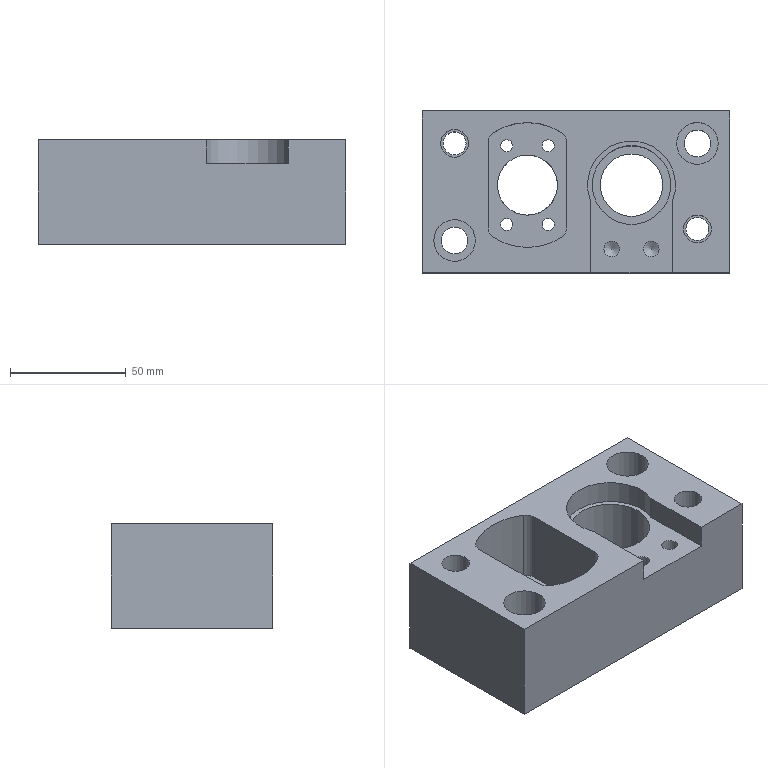Part | NX | features 26 2 | 1 solid | 43 faces | box 133 x 70 x 45 mm | volume 282044 mm3 | cylinder 24 | plane 17 | cone 2 | commonest cylinder face diameters 5.2 x4 10 x4 6.8 x2 10.001 x2 11.5 x2 12 x2
STEP:
#1=CARTESIAN_POINT('',(2251.6,-38.,-78.));
#2=VERTEX_POINT('',#1);
#3=CARTESIAN_POINT('',(2251.6,-7.158,-78.));
#4=VERTEX_POINT('',#3);
#5=CARTESIAN_POINT('',(2251.6,-13.,-78.));
#6=DIRECTION('',(0.,1.,0.));
#7=VECTOR('',#6,1000.);
#8=LINE('',#5,#7);
#9=EDGE_CURVE('',#2,#4,#8,.T.);
#10=ORIENTED_EDGE('',*,*,#9,.T.);
#11=CARTESIAN_POINT('',(2216.4,-7.158,-78.));
#12=VERTEX_POINT('',#11);
#13=CARTESIAN_POINT('',(2234.,0.,-78.));
#14=DIRECTION('',(0.,0.,1.));
#15=DIRECTION('',(-1.,0.,0.));
#16=AXIS2_PLACEMENT_3D('',#13,#14,#15);
#17=CIRCLE('',#16,19.);
#18=EDGE_CURVE('',#4,#12,#17,.T.);
#19=ORIENTED_EDGE('',*,*,#18,.T.);
#20=CARTESIAN_POINT('',(2216.4,-38.,-78.));
#21=VERTEX_POINT('',#20);
#22=CARTESIAN_POINT('',(2216.4,-13.,-78.));
#23=DIRECTION('',(0.,-1.,0.));
#24=VECTOR('',#23,1000.);
#25=LINE('',#22,#24);
#26=EDGE_CURVE('',#12,#21,#25,.T.);
#27=ORIENTED_EDGE('',*,*,#26,.T.);
#28=CARTESIAN_POINT('',(2234.,-38.,-78.));
#29=DIRECTION('',(1.,0.,0.));
#30=VECTOR('',#29,1000.);
#31=LINE('',#28,#30);
#32=EDGE_CURVE('',#21,#2,#31,.T.);
#33=ORIENTED_EDGE('',*,*,#32,.T.);
#34=EDGE_LOOP('',(#10,#19,#27,#33));
#35=FACE_BOUND('',#34,.T.);
#36=CARTESIAN_POINT('',(2239.1,-27.7,-78.));
#37=VERTEX_POINT('',#36);
#38=CARTESIAN_POINT('',(2242.5,-27.7,-78.));
#39=DIRECTION('',(0.,0.,-1.));
#40=DIRECTION('',(-1.,0.,0.));
#41=AXIS2_PLACEMENT_3D('',#38,#39,#40);
#42=CIRCLE('',#41,3.4);
#43=EDGE_CURVE('',#37,#37,#42,.T.);
#44=ORIENTED_EDGE('',*,*,#43,.T.);
#45=EDGE_LOOP('',(#44));
#46=FACE_BOUND('',#45,.T.);
#47=CARTESIAN_POINT('',(2222.1,-27.7,-78.));
#48=VERTEX_POINT('',#47);
#49=CARTESIAN_POINT('',(2225.5,-27.7,-78.));
#50=DIRECTION('',(0.,0.,1.));
#51=DIRECTION('',(-1.,0.,0.));
#52=AXIS2_PLACEMENT_3D('',#49,#50,#51);
#53=CIRCLE('',#52,3.4);
#54=EDGE_CURVE('',#48,#48,#53,.T.);
#55=ORIENTED_EDGE('',*,*,#54,.F.);
#56=EDGE_LOOP('',(#55));
#57=FACE_BOUND('',#56,.T.);
#58=CARTESIAN_POINT('',(2217.,0.,-78.));
#59=VERTEX_POINT('',#58);
#60=CARTESIAN_POINT('',(2234.,0.,-78.));
#61=DIRECTION('',(0.,0.,1.));
#62=DIRECTION('',(-1.,0.,0.));
#63=AXIS2_PLACEMENT_3D('',#60,#61,#62);
#64=CIRCLE('',#63,17.);
#65=EDGE_CURVE('',#59,#59,#64,.T.);
#66=ORIENTED_EDGE('',*,*,#65,.F.);
#67=EDGE_LOOP('',(#66));
#68=FACE_BOUND('',#67,.T.);
#69=CARTESIAN_POINT('',(2258.,-3.,-78.));
#70=DIRECTION('',(0.,0.,1.));
#71=DIRECTION('',(1.,0.,0.));
#72=AXIS2_PLACEMENT_3D('',#69,#70,#71);
#73=PLANE('',#72);
#74=ADVANCED_FACE('',(#35,#46,#57,#68),#73,.T.);
#75=CARTESIAN_POINT('',(2217.,0.,-108.));
#76=VERTEX_POINT('',#75);
#77=CARTESIAN_POINT('',(2234.,0.,-108.));
#78=DIRECTION('',(0.,0.,-1.));
#79=DIRECTION('',(-1.,0.,0.));
#80=AXIS2_PLACEMENT_3D('',#77,#78,#79);
#81=CIRCLE('',#80,17.);
#82=EDGE_CURVE('',#76,#76,#81,.T.);
#83=ORIENTED_EDGE('',*,*,#82,.T.);
#84=EDGE_LOOP('',(#83));
#85=FACE_BOUND('',#84,.T.);
#86=ORIENTED_EDGE('',*,*,#65,.T.);
#87=EDGE_LOOP('',(#86));
#88=FACE_BOUND('',#87,.T.);
#89=CARTESIAN_POINT('',(2234.,0.,512.));
#90=DIRECTION('',(0.,0.,-1.));
#91=DIRECTION('',(-1.,0.,0.));
#92=AXIS2_PLACEMENT_3D('',#89,#90,#91);
#93=CYLINDRICAL_SURFACE('',#92,17.);
#94=ADVANCED_FACE('',(#85,#88),#93,.F.);
#95=CARTESIAN_POINT('',(2151.5,18.,-68.));
#96=VERTEX_POINT('',#95);
#97=CARTESIAN_POINT('',(2157.5,18.,-68.));
#98=DIRECTION('',(0.,0.,1.));
#99=DIRECTION('',(-1.,0.,0.));
#100=AXIS2_PLACEMENT_3D('',#97,#98,#99);
#101=CIRCLE('',#100,6.);
#102=EDGE_CURVE('',#96,#96,#101,.T.);
#103=ORIENTED_EDGE('',*,*,#102,.F.);
#104=EDGE_LOOP('',(#103));
#105=FACE_BOUND('',#104,.T.);
#106=CARTESIAN_POINT('',(2256.5,-19.,-68.));
#107=VERTEX_POINT('',#106);
#108=CARTESIAN_POINT('',(2262.5,-19.,-68.));
#109=DIRECTION('',(0.,0.,1.));
#110=DIRECTION('',(-1.,0.,0.));
#111=AXIS2_PLACEMENT_3D('',#108,#109,#110);
#112=CIRCLE('',#111,6.);
#113=EDGE_CURVE('',#107,#107,#112,.T.);
#114=ORIENTED_EDGE('',*,*,#113,.F.);
#115=EDGE_LOOP('',(#114));
#116=FACE_BOUND('',#115,.T.);
#117=CARTESIAN_POINT('',(2253.5,18.,-68.));
#118=VERTEX_POINT('',#117);
#119=CARTESIAN_POINT('',(2262.5,18.,-68.));
#120=DIRECTION('',(0.,0.,-1.));
#121=DIRECTION('',(-1.,0.,0.));
#122=AXIS2_PLACEMENT_3D('',#119,#120,#121);
#123=CIRCLE('',#122,9.);
#124=EDGE_CURVE('',#118,#118,#123,.T.);
#125=ORIENTED_EDGE('',*,*,#124,.T.);
#126=EDGE_LOOP('',(#125));
#127=FACE_BOUND('',#126,.T.);
#128=CARTESIAN_POINT('',(2148.5,-24.,-68.));
#129=VERTEX_POINT('',#128);
#130=CARTESIAN_POINT('',(2157.5,-24.,-68.));
#131=DIRECTION('',(0.,0.,-1.));
#132=DIRECTION('',(-1.,0.,0.));
#133=AXIS2_PLACEMENT_3D('',#130,#131,#132);
#134=CIRCLE('',#133,9.);
#135=EDGE_CURVE('',#129,#129,#134,.T.);
#136=ORIENTED_EDGE('',*,*,#135,.T.);
#137=EDGE_LOOP('',(#136));
#138=FACE_BOUND('',#137,.T.);
#139=CARTESIAN_POINT('',(2206.,18.439,-68.));
#140=VERTEX_POINT('',#139);
#141=CARTESIAN_POINT('',(2206.,-18.439,-68.));
#142=VERTEX_POINT('',#141);
#143=CARTESIAN_POINT('',(2206.,211.,-68.));
#144=DIRECTION('',(0.,-1.,0.));
#145=VECTOR('',#144,1000.);
#146=LINE('',#143,#145);
#147=EDGE_CURVE('',#140,#142,#146,.T.);
#148=ORIENTED_EDGE('',*,*,#147,.T.);
#149=CARTESIAN_POINT('',(2203.727,-22.63,-68.));
#150=VERTEX_POINT('',#149);
#151=CARTESIAN_POINT('',(2201.,-18.439,-68.));
#152=DIRECTION('',(0.,0.,-1.));
#153=DIRECTION('',(-1.,0.,0.));
#154=AXIS2_PLACEMENT_3D('',#151,#152,#153);
#155=CIRCLE('',#154,5.);
#156=EDGE_CURVE('',#142,#150,#155,.T.);
#157=ORIENTED_EDGE('',*,*,#156,.T.);
#158=CARTESIAN_POINT('',(2174.273,-22.63,-68.));
#159=VERTEX_POINT('',#158);
#160=CARTESIAN_POINT('',(2189.,0.,-68.));
#161=DIRECTION('',(0.,0.,-1.));
#162=DIRECTION('',(-1.,0.,0.));
#163=AXIS2_PLACEMENT_3D('',#160,#161,#162);
#164=CIRCLE('',#163,27.);
#165=EDGE_CURVE('',#150,#159,#164,.T.);
#166=ORIENTED_EDGE('',*,*,#165,.T.);
#167=CARTESIAN_POINT('',(2172.,-18.439,-68.));
#168=VERTEX_POINT('',#167);
#169=CARTESIAN_POINT('',(2177.,-18.439,-68.));
#170=DIRECTION('',(0.,0.,-1.));
#171=DIRECTION('',(-1.,0.,0.));
#172=AXIS2_PLACEMENT_3D('',#169,#170,#171);
#173=CIRCLE('',#172,5.);
#174=EDGE_CURVE('',#159,#168,#173,.T.);
#175=ORIENTED_EDGE('',*,*,#174,.T.);
#176=CARTESIAN_POINT('',(2172.,18.439,-68.));
#177=VERTEX_POINT('',#176);
#178=CARTESIAN_POINT('',(2172.,211.,-68.));
#179=DIRECTION('',(0.,1.,0.));
#180=VECTOR('',#179,1000.);
#181=LINE('',#178,#180);
#182=EDGE_CURVE('',#168,#177,#181,.T.);
#183=ORIENTED_EDGE('',*,*,#182,.T.);
#184=CARTESIAN_POINT('',(2174.273,22.63,-68.));
#185=VERTEX_POINT('',#184);
#186=CARTESIAN_POINT('',(2177.,18.439,-68.));
#187=DIRECTION('',(0.,0.,-1.));
#188=DIRECTION('',(-1.,0.,0.));
#189=AXIS2_PLACEMENT_3D('',#186,#187,#188);
#190=CIRCLE('',#189,5.);
#191=EDGE_CURVE('',#177,#185,#190,.T.);
#192=ORIENTED_EDGE('',*,*,#191,.T.);
#193=CARTESIAN_POINT('',(2203.727,22.63,-68.));
#194=VERTEX_POINT('',#193);
#195=CARTESIAN_POINT('',(2189.,0.,-68.));
#196=DIRECTION('',(0.,0.,-1.));
#197=DIRECTION('',(-1.,0.,0.));
#198=AXIS2_PLACEMENT_3D('',#195,#196,#197);
#199=CIRCLE('',#198,27.);
#200=EDGE_CURVE('',#185,#194,#199,.T.);
#201=ORIENTED_EDGE('',*,*,#200,.T.);
#202=CARTESIAN_POINT('',(2201.,18.439,-68.));
#203=DIRECTION('',(0.,0.,-1.));
#204=DIRECTION('',(-1.,0.,0.));
#205=AXIS2_PLACEMENT_3D('',#202,#203,#204);
#206=CIRCLE('',#205,5.);
#207=EDGE_CURVE('',#194,#140,#206,.T.);
#208=ORIENTED_EDGE('',*,*,#207,.T.);
#209=EDGE_LOOP('',(#148,#157,#166,#175,#183,#192,#201,#208));
#210=FACE_BOUND('',#209,.T.);
#211=CARTESIAN_POINT('',(2216.4,-7.158,-68.));
#212=VERTEX_POINT('',#211);
#213=CARTESIAN_POINT('',(2251.6,-7.158,-68.));
#214=VERTEX_POINT('',#213);
#215=CARTESIAN_POINT('',(2234.,0.,-68.));
#216=DIRECTION('',(0.,0.,-1.));
#217=DIRECTION('',(1.,0.,0.));
#218=AXIS2_PLACEMENT_3D('',#215,#216,#217);
#219=CIRCLE('',#218,19.);
#220=EDGE_CURVE('',#212,#214,#219,.T.);
#221=ORIENTED_EDGE('',*,*,#220,.T.);
#222=CARTESIAN_POINT('',(2251.6,-38.,-68.));
#223=VERTEX_POINT('',#222);
#224=CARTESIAN_POINT('',(2251.6,206.,-68.));
#225=DIRECTION('',(0.,-1.,0.));
#226=VECTOR('',#225,1000.);
#227=LINE('',#224,#226);
#228=EDGE_CURVE('',#214,#223,#227,.T.);
#229=ORIENTED_EDGE('',*,*,#228,.T.);
#230=CARTESIAN_POINT('',(2276.5,-38.,-68.));
#231=VERTEX_POINT('',#230);
#232=CARTESIAN_POINT('',(2234.,-38.,-68.));
#233=DIRECTION('',(-1.,0.,0.));
#234=VECTOR('',#233,1000.);
#235=LINE('',#232,#234);
#236=EDGE_CURVE('',#231,#223,#235,.T.);
#237=ORIENTED_EDGE('',*,*,#236,.F.);
#238=CARTESIAN_POINT('',(2276.5,32.,-68.));
#239=VERTEX_POINT('',#238);
#240=CARTESIAN_POINT('',(2276.5,0.,-68.));
#241=DIRECTION('',(0.,-1.,0.));
#242=VECTOR('',#241,1000.);
#243=LINE('',#240,#242);
#244=EDGE_CURVE('',#239,#231,#243,.T.);
#245=ORIENTED_EDGE('',*,*,#244,.F.);
#246=CARTESIAN_POINT('',(2143.5,32.,-68.));
#247=VERTEX_POINT('',#246);
#248=CARTESIAN_POINT('',(2234.,32.,-68.));
#249=DIRECTION('',(1.,0.,0.));
#250=VECTOR('',#249,1000.);
#251=LINE('',#248,#250);
#252=EDGE_CURVE('',#247,#239,#251,.T.);
#253=ORIENTED_EDGE('',*,*,#252,.F.);
#254=CARTESIAN_POINT('',(2143.5,-38.,-68.));
#255=VERTEX_POINT('',#254);
#256=CARTESIAN_POINT('',(2143.5,0.,-68.));
#257=DIRECTION('',(0.,1.,0.));
#258=VECTOR('',#257,1000.);
#259=LINE('',#256,#258);
#260=EDGE_CURVE('',#255,#247,#259,.T.);
#261=ORIENTED_EDGE('',*,*,#260,.F.);
#262=CARTESIAN_POINT('',(2216.4,-38.,-68.));
#263=VERTEX_POINT('',#262);
#264=CARTESIAN_POINT('',(2234.,-38.,-68.));
#265=DIRECTION('',(-1.,0.,0.));
#266=VECTOR('',#265,1000.);
#267=LINE('',#264,#266);
#268=EDGE_CURVE('',#263,#255,#267,.T.);
#269=ORIENTED_EDGE('',*,*,#268,.F.);
#270=CARTESIAN_POINT('',(2216.4,206.,-68.));
#271=DIRECTION('',(0.,1.,0.));
#272=VECTOR('',#271,1000.);
#273=LINE('',#270,#272);
#274=EDGE_CURVE('',#263,#212,#273,.T.);
#275=ORIENTED_EDGE('',*,*,#274,.T.);
#276=EDGE_LOOP('',(#221,#229,#237,#245,#253,#261,#269,#275));
#277=FACE_BOUND('',#276,.T.);
#278=CARTESIAN_POINT('',(1069.5,206.,-68.));
#279=DIRECTION('',(0.,0.,-1.));
#280=DIRECTION('',(-1.,0.,0.));
#281=AXIS2_PLACEMENT_3D('',#278,#279,#280);
#282=PLANE('',#281);
#283=ADVANCED_FACE('',(#105,#116,#127,#138,#210,#277),#282,.F.);
#284=CARTESIAN_POINT('',(2276.5,-38.,-113.));
#285=VERTEX_POINT('',#284);
#286=CARTESIAN_POINT('',(2276.5,-38.,-123.5));
#287=DIRECTION('',(0.,0.,1.));
#288=VECTOR('',#287,1000.);
#289=LINE('',#286,#288);
#290=EDGE_CURVE('',#285,#231,#289,.T.);
#291=ORIENTED_EDGE('',*,*,#290,.F.);
#292=CARTESIAN_POINT('',(2276.5,32.,-113.));
#293=VERTEX_POINT('',#292);
#294=CARTESIAN_POINT('',(2276.5,0.,-113.));
#295=DIRECTION('',(0.,1.,0.));
#296=VECTOR('',#295,1000.);
#297=LINE('',#294,#296);
#298=EDGE_CURVE('',#285,#293,#297,.T.);
#299=ORIENTED_EDGE('',*,*,#298,.T.);
#300=CARTESIAN_POINT('',(2276.5,32.,-123.5));
#301=DIRECTION('',(0.,0.,1.));
#302=VECTOR('',#301,1000.);
#303=LINE('',#300,#302);
#304=EDGE_CURVE('',#293,#239,#303,.T.);
#305=ORIENTED_EDGE('',*,*,#304,.T.);
#306=ORIENTED_EDGE('',*,*,#244,.T.);
#307=EDGE_LOOP('',(#291,#299,#305,#306));
#308=FACE_BOUND('',#307,.T.);
#309=CARTESIAN_POINT('',(2276.5,0.,-123.5));
#310=DIRECTION('',(1.,0.,0.));
#311=DIRECTION('',(0.,0.,-1.));
#312=AXIS2_PLACEMENT_3D('',#309,#310,#311);
#313=PLANE('',#312);
#314=ADVANCED_FACE('',(#308),#313,.T.);
#315=ORIENTED_EDGE('',*,*,#304,.F.);
#316=CARTESIAN_POINT('',(2143.5,32.,-113.));
#317=VERTEX_POINT('',#316);
#318=CARTESIAN_POINT('',(2234.,32.,-113.));
#319=DIRECTION('',(-1.,0.,0.));
#320=VECTOR('',#319,1000.);
#321=LINE('',#318,#320);
#322=EDGE_CURVE('',#293,#317,#321,.T.);
#323=ORIENTED_EDGE('',*,*,#322,.T.);
#324=CARTESIAN_POINT('',(2143.5,32.,-123.5));
#325=DIRECTION('',(0.,0.,1.));
#326=VECTOR('',#325,1000.);
#327=LINE('',#324,#326);
#328=EDGE_CURVE('',#317,#247,#327,.T.);
#329=ORIENTED_EDGE('',*,*,#328,.T.);
#330=ORIENTED_EDGE('',*,*,#252,.T.);
#331=EDGE_LOOP('',(#315,#323,#329,#330));
#332=FACE_BOUND('',#331,.T.);
#333=CARTESIAN_POINT('',(2234.,32.,-123.5));
#334=DIRECTION('',(0.,1.,0.));
#335=DIRECTION('',(0.,0.,1.));
#336=AXIS2_PLACEMENT_3D('',#333,#334,#335);
#337=PLANE('',#336);
#338=ADVANCED_FACE('',(#332),#337,.T.);
#339=ORIENTED_EDGE('',*,*,#328,.F.);
#340=CARTESIAN_POINT('',(2143.5,-38.,-113.));
#341=VERTEX_POINT('',#340);
#342=CARTESIAN_POINT('',(2143.5,0.,-113.));
#343=DIRECTION('',(0.,-1.,0.));
#344=VECTOR('',#343,1000.);
#345=LINE('',#342,#344);
#346=EDGE_CURVE('',#317,#341,#345,.T.);
#347=ORIENTED_EDGE('',*,*,#346,.T.);
#348=CARTESIAN_POINT('',(2143.5,-38.,-123.5));
#349=DIRECTION('',(0.,0.,1.));
#350=VECTOR('',#349,1000.);
#351=LINE('',#348,#350);
#352=EDGE_CURVE('',#341,#255,#351,.T.);
#353=ORIENTED_EDGE('',*,*,#352,.T.);
#354=ORIENTED_EDGE('',*,*,#260,.T.);
#355=EDGE_LOOP('',(#339,#347,#353,#354));
#356=FACE_BOUND('',#355,.T.);
#357=CARTESIAN_POINT('',(2143.5,0.,-123.5));
#358=DIRECTION('',(-1.,0.,0.));
#359=DIRECTION('',(0.,0.,1.));
#360=AXIS2_PLACEMENT_3D('',#357,#358,#359);
#361=PLANE('',#360);
#362=ADVANCED_FACE('',(#356),#361,.T.);
#363=ORIENTED_EDGE('',*,*,#32,.F.);
#364=CARTESIAN_POINT('',(2216.4,-38.,-123.5));
#365=DIRECTION('',(0.,0.,-1.));
#366=VECTOR('',#365,1000.);
#367=LINE('',#364,#366);
#368=EDGE_CURVE('',#263,#21,#367,.T.);
#369=ORIENTED_EDGE('',*,*,#368,.F.);
#370=ORIENTED_EDGE('',*,*,#268,.T.);
#371=ORIENTED_EDGE('',*,*,#352,.F.);
#372=CARTESIAN_POINT('',(2234.,-38.,-113.));
#373=DIRECTION('',(1.,0.,0.));
#374=VECTOR('',#373,1000.);
#375=LINE('',#372,#374);
#376=EDGE_CURVE('',#341,#285,#375,.T.);
#377=ORIENTED_EDGE('',*,*,#376,.T.);
#378=ORIENTED_EDGE('',*,*,#290,.T.);
#379=ORIENTED_EDGE('',*,*,#236,.T.);
#380=CARTESIAN_POINT('',(2251.6,-38.,-58.));
#381=DIRECTION('',(0.,0.,-1.));
#382=VECTOR('',#381,1000.);
#383=LINE('',#380,#382);
#384=EDGE_CURVE('',#223,#2,#383,.T.);
#385=ORIENTED_EDGE('',*,*,#384,.T.);
#386=EDGE_LOOP('',(#363,#369,#370,#371,#377,#378,#379,#385));
#387=FACE_BOUND('',#386,.T.);
#388=CARTESIAN_POINT('',(2234.,-38.,-123.5));
#389=DIRECTION('',(0.,-1.,0.));
#390=DIRECTION('',(0.,0.,-1.));
#391=AXIS2_PLACEMENT_3D('',#388,#389,#390);
#392=PLANE('',#391);
#393=ADVANCED_FACE('',(#387),#392,.T.);
#394=CARTESIAN_POINT('',(2257.499,-19.,-88.5));
#395=VERTEX_POINT('',#394);
#396=CARTESIAN_POINT('',(2262.5,-19.,-88.5));
#397=DIRECTION('',(0.,0.,-1.));
#398=DIRECTION('',(-1.,0.,0.));
#399=AXIS2_PLACEMENT_3D('',#396,#397,#398);
#400=CIRCLE('',#399,5.);
#401=EDGE_CURVE('',#395,#395,#400,.T.);
#402=ORIENTED_EDGE('',*,*,#401,.F.);
#403=EDGE_LOOP('',(#402));
#404=FACE_BOUND('',#403,.T.);
#405=CARTESIAN_POINT('',(2257.499,-19.,-113.));
#406=VERTEX_POINT('',#405);
#407=CARTESIAN_POINT('',(2262.5,-19.,-113.));
#408=DIRECTION('',(0.,0.,1.));
#409=DIRECTION('',(-1.,0.,0.));
#410=AXIS2_PLACEMENT_3D('',#407,#408,#409);
#411=CIRCLE('',#410,5.);
#412=EDGE_CURVE('',#406,#406,#411,.T.);
#413=ORIENTED_EDGE('',*,*,#412,.F.);
#414=EDGE_LOOP('',(#413));
#415=FACE_BOUND('',#414,.T.);
#416=CARTESIAN_POINT('',(2262.5,-19.,541.5));
#417=DIRECTION('',(0.,0.,-1.));
#418=DIRECTION('',(-1.,0.,0.));
#419=AXIS2_PLACEMENT_3D('',#416,#417,#418);
#420=CYLINDRICAL_SURFACE('',#419,5.);
#421=ADVANCED_FACE('',(#404,#415),#420,.F.);
#422=CARTESIAN_POINT('',(2152.499,18.,-88.5));
#423=VERTEX_POINT('',#422);
#424=CARTESIAN_POINT('',(2157.5,18.,-88.5));
#425=DIRECTION('',(0.,0.,-1.));
#426=DIRECTION('',(-1.,0.,0.));
#427=AXIS2_PLACEMENT_3D('',#424,#425,#426);
#428=CIRCLE('',#427,5.);
#429=EDGE_CURVE('',#423,#423,#428,.T.);
#430=ORIENTED_EDGE('',*,*,#429,.F.);
#431=EDGE_LOOP('',(#430));
#432=FACE_BOUND('',#431,.T.);
#433=CARTESIAN_POINT('',(2152.499,18.,-113.));
#434=VERTEX_POINT('',#433);
#435=CARTESIAN_POINT('',(2157.5,18.,-113.));
#436=DIRECTION('',(0.,0.,1.));
#437=DIRECTION('',(-1.,0.,0.));
#438=AXIS2_PLACEMENT_3D('',#435,#436,#437);
#439=CIRCLE('',#438,5.);
#440=EDGE_CURVE('',#434,#434,#439,.T.);
#441=ORIENTED_EDGE('',*,*,#440,.F.);
#442=EDGE_LOOP('',(#441));
#443=FACE_BOUND('',#442,.T.);
#444=CARTESIAN_POINT('',(2157.5,18.,541.5));
#445=DIRECTION('',(0.,0.,-1.));
#446=DIRECTION('',(-1.,0.,0.));
#447=AXIS2_PLACEMENT_3D('',#444,#445,#446);
#448=CYLINDRICAL_SURFACE('',#447,5.);
#449=ADVANCED_FACE('',(#432,#443),#448,.F.);
#450=CARTESIAN_POINT('',(2256.75,18.,-88.5));
#451=VERTEX_POINT('',#450);
#452=CARTESIAN_POINT('',(2262.5,18.,-88.5));
#453=DIRECTION('',(0.,0.,-1.));
#454=DIRECTION('',(-1.,0.,0.));
#455=AXIS2_PLACEMENT_3D('',#452,#453,#454);
#456=CIRCLE('',#455,5.75);
#457=EDGE_CURVE('',#451,#451,#456,.T.);
#458=ORIENTED_EDGE('',*,*,#457,.F.);
#459=EDGE_LOOP('',(#458));
#460=FACE_BOUND('',#459,.T.);
#461=CARTESIAN_POINT('',(2256.75,18.,-113.));
#462=VERTEX_POINT('',#461);
#463=CARTESIAN_POINT('',(2262.5,18.,-113.));
#464=DIRECTION('',(0.,0.,1.));
#465=DIRECTION('',(-1.,0.,0.));
#466=AXIS2_PLACEMENT_3D('',#463,#464,#465);
#467=CIRCLE('',#466,5.75);
#468=EDGE_CURVE('',#462,#462,#467,.T.);
#469=ORIENTED_EDGE('',*,*,#468,.F.);
#470=EDGE_LOOP('',(#469));
#471=FACE_BOUND('',#470,.T.);
#472=CARTESIAN_POINT('',(2262.5,18.,-66.5));
#473=DIRECTION('',(0.,0.,-1.));
#474=DIRECTION('',(1.,0.,0.));
#475=AXIS2_PLACEMENT_3D('',#472,#473,#474);
#476=CYLINDRICAL_SURFACE('',#475,5.75);
#477=ADVANCED_FACE('',(#460,#471),#476,.F.);
#478=CARTESIAN_POINT('',(2151.75,-24.,-88.5));
#479=VERTEX_POINT('',#478);
#480=CARTESIAN_POINT('',(2157.5,-24.,-88.5));
#481=DIRECTION('',(0.,0.,-1.));
#482=DIRECTION('',(-1.,0.,0.));
#483=AXIS2_PLACEMENT_3D('',#480,#481,#482);
#484=CIRCLE('',#483,5.75);
#485=EDGE_CURVE('',#479,#479,#484,.T.);
#486=ORIENTED_EDGE('',*,*,#485,.F.);
#487=EDGE_LOOP('',(#486));
#488=FACE_BOUND('',#487,.T.);
#489=CARTESIAN_POINT('',(2151.75,-24.,-113.));
#490=VERTEX_POINT('',#489);
#491=CARTESIAN_POINT('',(2157.5,-24.,-113.));
#492=DIRECTION('',(0.,0.,1.));
#493=DIRECTION('',(-1.,0.,0.));
#494=AXIS2_PLACEMENT_3D('',#491,#492,#493);
#495=CIRCLE('',#494,5.75);
#496=EDGE_CURVE('',#490,#490,#495,.T.);
#497=ORIENTED_EDGE('',*,*,#496,.F.);
#498=EDGE_LOOP('',(#497));
#499=FACE_BOUND('',#498,.T.);
#500=CARTESIAN_POINT('',(2157.5,-24.,-66.5));
#501=DIRECTION('',(0.,0.,-1.));
#502=DIRECTION('',(1.,0.,0.));
#503=AXIS2_PLACEMENT_3D('',#500,#501,#502);
#504=CYLINDRICAL_SURFACE('',#503,5.75);
#505=ADVANCED_FACE('',(#488,#499),#504,.F.);
#506=CARTESIAN_POINT('',(2220.5,0.,-108.));
#507=VERTEX_POINT('',#506);
#508=CARTESIAN_POINT('',(2234.,0.,-108.));
#509=DIRECTION('',(0.,0.,-1.));
#510=DIRECTION('',(-1.,0.,0.));
#511=AXIS2_PLACEMENT_3D('',#508,#509,#510);
#512=CIRCLE('',#511,13.5);
#513=EDGE_CURVE('',#507,#507,#512,.T.);
#514=ORIENTED_EDGE('',*,*,#513,.F.);
#515=EDGE_LOOP('',(#514));
#516=FACE_BOUND('',#515,.T.);
#517=CARTESIAN_POINT('',(2247.5,0.,-113.));
#518=VERTEX_POINT('',#517);
#519=CARTESIAN_POINT('',(2234.,0.,-113.));
#520=DIRECTION('',(0.,0.,1.));
#521=DIRECTION('',(1.,0.,0.));
#522=AXIS2_PLACEMENT_3D('',#519,#520,#521);
#523=CIRCLE('',#522,13.5);
#524=EDGE_CURVE('',#518,#518,#523,.T.);
#525=ORIENTED_EDGE('',*,*,#524,.F.);
#526=EDGE_LOOP('',(#525));
#527=FACE_BOUND('',#526,.T.);
#528=CARTESIAN_POINT('',(2234.,0.,542.));
#529=DIRECTION('',(0.,0.,-1.));
#530=DIRECTION('',(-1.,0.,0.));
#531=AXIS2_PLACEMENT_3D('',#528,#529,#530);
#532=CYLINDRICAL_SURFACE('',#531,13.5);
#533=ADVANCED_FACE('',(#516,#527),#532,.F.);
#534=CARTESIAN_POINT('',(2163.5,18.,-88.5));
#535=VERTEX_POINT('',#534);
#536=CARTESIAN_POINT('',(2157.5,18.,-88.5));
#537=DIRECTION('',(0.,0.,1.));
#538=DIRECTION('',(1.,0.,0.));
#539=AXIS2_PLACEMENT_3D('',#536,#537,#538);
#540=CIRCLE('',#539,6.);
#541=EDGE_CURVE('',#535,#535,#540,.T.);
#542=ORIENTED_EDGE('',*,*,#541,.F.);
#543=EDGE_LOOP('',(#542));
#544=FACE_BOUND('',#543,.T.);
#545=ORIENTED_EDGE('',*,*,#102,.T.);
#546=EDGE_LOOP('',(#545));
#547=FACE_BOUND('',#546,.T.);
#548=CARTESIAN_POINT('',(2157.5,18.,541.5));
#549=DIRECTION('',(0.,0.,-1.));
#550=DIRECTION('',(-1.,0.,0.));
#551=AXIS2_PLACEMENT_3D('',#548,#549,#550);
#552=CYLINDRICAL_SURFACE('',#551,6.);
#553=ADVANCED_FACE('',(#544,#547),#552,.F.);
#554=CARTESIAN_POINT('',(2268.5,-19.,-88.5));
#555=VERTEX_POINT('',#554);
#556=CARTESIAN_POINT('',(2262.5,-19.,-88.5));
#557=DIRECTION('',(0.,0.,1.));
#558=DIRECTION('',(1.,0.,0.));
#559=AXIS2_PLACEMENT_3D('',#556,#557,#558);
#560=CIRCLE('',#559,6.);
#561=EDGE_CURVE('',#555,#555,#560,.T.);
#562=ORIENTED_EDGE('',*,*,#561,.F.);
#563=EDGE_LOOP('',(#562));
#564=FACE_BOUND('',#563,.T.);
#565=ORIENTED_EDGE('',*,*,#113,.T.);
#566=EDGE_LOOP('',(#565));
#567=FACE_BOUND('',#566,.T.);
#568=CARTESIAN_POINT('',(2262.5,-19.,541.5));
#569=DIRECTION('',(0.,0.,-1.));
#570=DIRECTION('',(-1.,0.,0.));
#571=AXIS2_PLACEMENT_3D('',#568,#569,#570);
#572=CYLINDRICAL_SURFACE('',#571,6.);
#573=ADVANCED_FACE('',(#564,#567),#572,.F.);
#574=CARTESIAN_POINT('',(2253.5,18.,-88.5));
#575=VERTEX_POINT('',#574);
#576=CARTESIAN_POINT('',(2262.5,18.,-88.5));
#577=DIRECTION('',(0.,0.,-1.));
#578=DIRECTION('',(-1.,0.,0.));
#579=AXIS2_PLACEMENT_3D('',#576,#577,#578);
#580=CIRCLE('',#579,9.);
#581=EDGE_CURVE('',#575,#575,#580,.T.);
#582=ORIENTED_EDGE('',*,*,#581,.T.);
#583=EDGE_LOOP('',(#582));
#584=FACE_BOUND('',#583,.T.);
#585=ORIENTED_EDGE('',*,*,#124,.F.);
#586=EDGE_LOOP('',(#585));
#587=FACE_BOUND('',#586,.T.);
#588=CARTESIAN_POINT('',(2262.5,18.,-68.5));
#589=DIRECTION('',(0.,0.,-1.));
#590=DIRECTION('',(1.,0.,0.));
#591=AXIS2_PLACEMENT_3D('',#588,#589,#590);
#592=CYLINDRICAL_SURFACE('',#591,9.);
#593=ADVANCED_FACE('',(#584,#587),#592,.F.);
#594=CARTESIAN_POINT('',(2148.5,-24.,-88.5));
#595=VERTEX_POINT('',#594);
#596=CARTESIAN_POINT('',(2157.5,-24.,-88.5));
#597=DIRECTION('',(0.,0.,-1.));
#598=DIRECTION('',(-1.,0.,0.));
#599=AXIS2_PLACEMENT_3D('',#596,#597,#598);
#600=CIRCLE('',#599,9.);
#601=EDGE_CURVE('',#595,#595,#600,.T.);
#602=ORIENTED_EDGE('',*,*,#601,.T.);
#603=EDGE_LOOP('',(#602));
#604=FACE_BOUND('',#603,.T.);
#605=ORIENTED_EDGE('',*,*,#135,.F.);
#606=EDGE_LOOP('',(#605));
#607=FACE_BOUND('',#606,.T.);
#608=CARTESIAN_POINT('',(2157.5,-24.,-68.5));
#609=DIRECTION('',(0.,0.,-1.));
#610=DIRECTION('',(1.,0.,0.));
#611=AXIS2_PLACEMENT_3D('',#608,#609,#610);
#612=CYLINDRICAL_SURFACE('',#611,9.);
#613=ADVANCED_FACE('',(#604,#607),#612,.F.);
#614=ORIENTED_EDGE('',*,*,#601,.F.);
#615=EDGE_LOOP('',(#614));
#616=FACE_BOUND('',#615,.T.);
#617=ORIENTED_EDGE('',*,*,#485,.T.);
#618=EDGE_LOOP('',(#617));
#619=FACE_BOUND('',#618,.T.);
#620=CARTESIAN_POINT('',(2214.5,18.,-88.5));
#621=DIRECTION('',(0.,0.,-1.));
#622=DIRECTION('',(-1.,0.,0.));
#623=AXIS2_PLACEMENT_3D('',#620,#621,#622);
#624=PLANE('',#623);
#625=ADVANCED_FACE('',(#616,#619),#624,.F.);
#626=ORIENTED_EDGE('',*,*,#541,.T.);
#627=EDGE_LOOP('',(#626));
#628=FACE_BOUND('',#627,.T.);
#629=ORIENTED_EDGE('',*,*,#429,.T.);
#630=EDGE_LOOP('',(#629));
#631=FACE_BOUND('',#630,.T.);
#632=CARTESIAN_POINT('',(2214.5,18.,-88.5));
#633=DIRECTION('',(0.,0.,-1.));
#634=DIRECTION('',(-1.,0.,0.));
#635=AXIS2_PLACEMENT_3D('',#632,#633,#634);
#636=PLANE('',#635);
#637=ADVANCED_FACE('',(#628,#631),#636,.F.);
#638=ORIENTED_EDGE('',*,*,#561,.T.);
#639=EDGE_LOOP('',(#638));
#640=FACE_BOUND('',#639,.T.);
#641=ORIENTED_EDGE('',*,*,#401,.T.);
#642=EDGE_LOOP('',(#641));
#643=FACE_BOUND('',#642,.T.);
#644=CARTESIAN_POINT('',(2262.5,23.,-88.5));
#645=DIRECTION('',(0.,0.,-1.));
#646=DIRECTION('',(-1.,0.,0.));
#647=AXIS2_PLACEMENT_3D('',#644,#645,#646);
#648=PLANE('',#647);
#649=ADVANCED_FACE('',(#640,#643),#648,.F.);
#650=ORIENTED_EDGE('',*,*,#82,.F.);
#651=EDGE_LOOP('',(#650));
#652=FACE_BOUND('',#651,.T.);
#653=ORIENTED_EDGE('',*,*,#513,.T.);
#654=EDGE_LOOP('',(#653));
#655=FACE_BOUND('',#654,.T.);
#656=CARTESIAN_POINT('',(2234.,0.,-108.));
#657=DIRECTION('',(0.,0.,1.));
#658=DIRECTION('',(1.,0.,0.));
#659=AXIS2_PLACEMENT_3D('',#656,#657,#658);
#660=PLANE('',#659);
#661=ADVANCED_FACE('',(#652,#655),#660,.T.);
#662=ORIENTED_EDGE('',*,*,#581,.F.);
#663=EDGE_LOOP('',(#662));
#664=FACE_BOUND('',#663,.T.);
#665=ORIENTED_EDGE('',*,*,#457,.T.);
#666=EDGE_LOOP('',(#665));
#667=FACE_BOUND('',#666,.T.);
#668=CARTESIAN_POINT('',(2262.5,18.,-88.5));
#669=DIRECTION('',(0.,0.,-1.));
#670=DIRECTION('',(-1.,0.,0.));
#671=AXIS2_PLACEMENT_3D('',#668,#669,#670);
#672=PLANE('',#671);
#673=ADVANCED_FACE('',(#664,#667),#672,.F.);
#674=CARTESIAN_POINT('',(2195.4,17.,-113.));
#675=VERTEX_POINT('',#674);
#676=CARTESIAN_POINT('',(2198.,17.,-113.));
#677=DIRECTION('',(0.,0.,-1.));
#678=DIRECTION('',(-1.,0.,0.));
#679=AXIS2_PLACEMENT_3D('',#676,#677,#678);
#680=CIRCLE('',#679,2.6);
#681=EDGE_CURVE('',#675,#675,#680,.T.);
#682=ORIENTED_EDGE('',*,*,#681,.F.);
#683=EDGE_LOOP('',(#682));
#684=FACE_BOUND('',#683,.T.);
#685=CARTESIAN_POINT('',(2195.4,-17.,-113.));
#686=VERTEX_POINT('',#685);
#687=CARTESIAN_POINT('',(2198.,-17.,-113.));
#688=DIRECTION('',(0.,0.,-1.));
#689=DIRECTION('',(-1.,0.,0.));
#690=AXIS2_PLACEMENT_3D('',#687,#688,#689);
#691=CIRCLE('',#690,2.6);
#692=EDGE_CURVE('',#686,#686,#691,.T.);
#693=ORIENTED_EDGE('',*,*,#692,.F.);
#694=EDGE_LOOP('',(#693));
#695=FACE_BOUND('',#694,.T.);
#696=CARTESIAN_POINT('',(2177.4,17.,-113.));
#697=VERTEX_POINT('',#696);
#698=CARTESIAN_POINT('',(2180.,17.,-113.));
#699=DIRECTION('',(0.,0.,-1.));
#700=DIRECTION('',(-1.,0.,0.));
#701=AXIS2_PLACEMENT_3D('',#698,#699,#700);
#702=CIRCLE('',#701,2.6);
#703=EDGE_CURVE('',#697,#697,#702,.T.);
#704=ORIENTED_EDGE('',*,*,#703,.F.);
#705=EDGE_LOOP('',(#704));
#706=FACE_BOUND('',#705,.T.);
#707=CARTESIAN_POINT('',(2177.4,-17.,-113.));
#708=VERTEX_POINT('',#707);
#709=CARTESIAN_POINT('',(2180.,-17.,-113.));
#710=DIRECTION('',(0.,0.,-1.));
#711=DIRECTION('',(-1.,0.,0.));
#712=AXIS2_PLACEMENT_3D('',#709,#710,#711);
#713=CIRCLE('',#712,2.6);
#714=EDGE_CURVE('',#708,#708,#713,.T.);
#715=ORIENTED_EDGE('',*,*,#714,.F.);
#716=EDGE_LOOP('',(#715));
#717=FACE_BOUND('',#716,.T.);
#718=CARTESIAN_POINT('',(2176.,0.,-113.));
#719=VERTEX_POINT('',#718);
#720=CARTESIAN_POINT('',(2189.,0.,-113.));
#721=DIRECTION('',(0.,0.,-1.));
#722=DIRECTION('',(-1.,0.,0.));
#723=AXIS2_PLACEMENT_3D('',#720,#721,#722);
#724=CIRCLE('',#723,13.);
#725=EDGE_CURVE('',#719,#719,#724,.T.);
#726=ORIENTED_EDGE('',*,*,#725,.F.);
#727=EDGE_LOOP('',(#726));
#728=FACE_BOUND('',#727,.T.);
#729=ORIENTED_EDGE('',*,*,#298,.F.);
#730=ORIENTED_EDGE('',*,*,#376,.F.);
#731=ORIENTED_EDGE('',*,*,#346,.F.);
#732=ORIENTED_EDGE('',*,*,#322,.F.);
#733=EDGE_LOOP('',(#729,#730,#731,#732));
#734=FACE_BOUND('',#733,.T.);
#735=ORIENTED_EDGE('',*,*,#440,.T.);
#736=EDGE_LOOP('',(#735));
#737=FACE_BOUND('',#736,.T.);
#738=ORIENTED_EDGE('',*,*,#496,.T.);
#739=EDGE_LOOP('',(#738));
#740=FACE_BOUND('',#739,.T.);
#741=ORIENTED_EDGE('',*,*,#524,.T.);
#742=EDGE_LOOP('',(#741));
#743=FACE_BOUND('',#742,.T.);
#744=ORIENTED_EDGE('',*,*,#468,.T.);
#745=EDGE_LOOP('',(#744));
#746=FACE_BOUND('',#745,.T.);
#747=ORIENTED_EDGE('',*,*,#412,.T.);
#748=EDGE_LOOP('',(#747));
#749=FACE_BOUND('',#748,.T.);
#750=CARTESIAN_POINT('',(1004.,-3.,-113.));
#751=DIRECTION('',(0.,0.,-1.));
#752=DIRECTION('',(1.,0.,0.));
#753=AXIS2_PLACEMENT_3D('',#750,#751,#752);
#754=PLANE('',#753);
#755=ADVANCED_FACE('',(#684,#695,#706,#717,#728,#734,#737,#740,#743,#746,#749),#754,.T.);
#756=CARTESIAN_POINT('',(2189.,13.,-100.));
#757=VERTEX_POINT('',#756);
#758=CARTESIAN_POINT('',(2189.,0.,-100.));
#759=DIRECTION('',(0.,0.,1.));
#760=DIRECTION('',(0.,1.,0.));
#761=AXIS2_PLACEMENT_3D('',#758,#759,#760);
#762=CIRCLE('',#761,13.);
#763=EDGE_CURVE('',#757,#757,#762,.T.);
#764=ORIENTED_EDGE('',*,*,#763,.T.);
#765=EDGE_LOOP('',(#764));
#766=FACE_BOUND('',#765,.T.);
#767=ORIENTED_EDGE('',*,*,#725,.T.);
#768=EDGE_LOOP('',(#767));
#769=FACE_BOUND('',#768,.T.);
#770=CARTESIAN_POINT('',(2189.,0.,-95.5));
#771=DIRECTION('',(0.,0.,1.));
#772=DIRECTION('',(1.,0.,0.));
#773=AXIS2_PLACEMENT_3D('',#770,#771,#772);
#774=CYLINDRICAL_SURFACE('',#773,13.);
#775=ADVANCED_FACE('',(#766,#769),#774,.F.);
#776=ORIENTED_EDGE('',*,*,#165,.F.);
#777=CARTESIAN_POINT('',(2203.727,-22.63,-100.));
#778=VERTEX_POINT('',#777);
#779=CARTESIAN_POINT('',(2203.727,-22.63,-95.5));
#780=DIRECTION('',(0.,0.,-1.));
#781=VECTOR('',#780,1000.);
#782=LINE('',#779,#781);
#783=EDGE_CURVE('',#150,#778,#782,.T.);
#784=ORIENTED_EDGE('',*,*,#783,.T.);
#785=CARTESIAN_POINT('',(2174.273,-22.63,-100.));
#786=VERTEX_POINT('',#785);
#787=CARTESIAN_POINT('',(2189.,0.,-100.));
#788=DIRECTION('',(0.,0.,1.));
#789=DIRECTION('',(0.,1.,0.));
#790=AXIS2_PLACEMENT_3D('',#787,#788,#789);
#791=CIRCLE('',#790,27.);
#792=EDGE_CURVE('',#786,#778,#791,.T.);
#793=ORIENTED_EDGE('',*,*,#792,.F.);
#794=CARTESIAN_POINT('',(2174.273,-22.63,-95.5));
#795=DIRECTION('',(0.,0.,1.));
#796=VECTOR('',#795,1000.);
#797=LINE('',#794,#796);
#798=EDGE_CURVE('',#786,#159,#797,.T.);
#799=ORIENTED_EDGE('',*,*,#798,.T.);
#800=EDGE_LOOP('',(#776,#784,#793,#799));
#801=FACE_BOUND('',#800,.T.);
#802=CARTESIAN_POINT('',(2189.,0.,-95.5));
#803=DIRECTION('',(0.,0.,1.));
#804=DIRECTION('',(1.,0.,0.));
#805=AXIS2_PLACEMENT_3D('',#802,#803,#804);
#806=CYLINDRICAL_SURFACE('',#805,27.);
#807=ADVANCED_FACE('',(#801),#806,.F.);
#808=CARTESIAN_POINT('',(2172.,18.439,-100.));
#809=VERTEX_POINT('',#808);
#810=CARTESIAN_POINT('',(2172.,-18.439,-100.));
#811=VERTEX_POINT('',#810);
#812=CARTESIAN_POINT('',(2172.,0.,-100.));
#813=DIRECTION('',(0.,-1.,0.));
#814=VECTOR('',#813,1000.);
#815=LINE('',#812,#814);
#816=EDGE_CURVE('',#809,#811,#815,.T.);
#817=ORIENTED_EDGE('',*,*,#816,.F.);
#818=CARTESIAN_POINT('',(2172.,18.439,-68.5));
#819=DIRECTION('',(0.,0.,1.));
#820=VECTOR('',#819,1000.);
#821=LINE('',#818,#820);
#822=EDGE_CURVE('',#809,#177,#821,.T.);
#823=ORIENTED_EDGE('',*,*,#822,.T.);
#824=ORIENTED_EDGE('',*,*,#182,.F.);
#825=CARTESIAN_POINT('',(2172.,-18.439,-100.));
#826=DIRECTION('',(0.,0.,-1.));
#827=VECTOR('',#826,1000.);
#828=LINE('',#825,#827);
#829=EDGE_CURVE('',#168,#811,#828,.T.);
#830=ORIENTED_EDGE('',*,*,#829,.T.);
#831=EDGE_LOOP('',(#817,#823,#824,#830));
#832=FACE_BOUND('',#831,.T.);
#833=CARTESIAN_POINT('',(2172.,0.,-95.5));
#834=DIRECTION('',(-1.,0.,0.));
#835=DIRECTION('',(0.,-1.,0.));
#836=AXIS2_PLACEMENT_3D('',#833,#834,#835);
#837=PLANE('',#836);
#838=ADVANCED_FACE('',(#832),#837,.F.);
#839=ORIENTED_EDGE('',*,*,#200,.F.);
#840=CARTESIAN_POINT('',(2174.273,22.63,-100.));
#841=VERTEX_POINT('',#840);
#842=CARTESIAN_POINT('',(2174.273,22.63,-95.5));
#843=DIRECTION('',(0.,0.,-1.));
#844=VECTOR('',#843,1000.);
#845=LINE('',#842,#844);
#846=EDGE_CURVE('',#185,#841,#845,.T.);
#847=ORIENTED_EDGE('',*,*,#846,.T.);
#848=CARTESIAN_POINT('',(2203.727,22.63,-100.));
#849=VERTEX_POINT('',#848);
#850=CARTESIAN_POINT('',(2189.,0.,-100.));
#851=DIRECTION('',(0.,0.,1.));
#852=DIRECTION('',(0.,1.,0.));
#853=AXIS2_PLACEMENT_3D('',#850,#851,#852);
#854=CIRCLE('',#853,27.);
#855=EDGE_CURVE('',#849,#841,#854,.T.);
#856=ORIENTED_EDGE('',*,*,#855,.F.);
#857=CARTESIAN_POINT('',(2203.727,22.63,-95.5));
#858=DIRECTION('',(0.,0.,1.));
#859=VECTOR('',#858,1000.);
#860=LINE('',#857,#859);
#861=EDGE_CURVE('',#849,#194,#860,.T.);
#862=ORIENTED_EDGE('',*,*,#861,.T.);
#863=EDGE_LOOP('',(#839,#847,#856,#862));
#864=FACE_BOUND('',#863,.T.);
#865=CARTESIAN_POINT('',(2189.,0.,-95.5));
#866=DIRECTION('',(0.,0.,1.));
#867=DIRECTION('',(1.,0.,0.));
#868=AXIS2_PLACEMENT_3D('',#865,#866,#867);
#869=CYLINDRICAL_SURFACE('',#868,27.);
#870=ADVANCED_FACE('',(#864),#869,.F.);
#871=ORIENTED_EDGE('',*,*,#147,.F.);
#872=CARTESIAN_POINT('',(2206.,18.439,-100.));
#873=VERTEX_POINT('',#872);
#874=CARTESIAN_POINT('',(2206.,18.439,-100.));
#875=DIRECTION('',(0.,0.,-1.));
#876=VECTOR('',#875,1000.);
#877=LINE('',#874,#876);
#878=EDGE_CURVE('',#140,#873,#877,.T.);
#879=ORIENTED_EDGE('',*,*,#878,.T.);
#880=CARTESIAN_POINT('',(2206.,-18.439,-100.));
#881=VERTEX_POINT('',#880);
#882=CARTESIAN_POINT('',(2206.,0.,-100.));
#883=DIRECTION('',(0.,1.,0.));
#884=VECTOR('',#883,1000.);
#885=LINE('',#882,#884);
#886=EDGE_CURVE('',#881,#873,#885,.T.);
#887=ORIENTED_EDGE('',*,*,#886,.F.);
#888=CARTESIAN_POINT('',(2206.,-18.439,-68.5));
#889=DIRECTION('',(0.,0.,1.));
#890=VECTOR('',#889,1000.);
#891=LINE('',#888,#890);
#892=EDGE_CURVE('',#881,#142,#891,.T.);
#893=ORIENTED_EDGE('',*,*,#892,.T.);
#894=EDGE_LOOP('',(#871,#879,#887,#893));
#895=FACE_BOUND('',#894,.T.);
#896=CARTESIAN_POINT('',(2206.,0.,-95.5));
#897=DIRECTION('',(1.,0.,0.));
#898=DIRECTION('',(0.,1.,0.));
#899=AXIS2_PLACEMENT_3D('',#896,#897,#898);
#900=PLANE('',#899);
#901=ADVANCED_FACE('',(#895),#900,.F.);
#902=CARTESIAN_POINT('',(2200.6,17.,-100.));
#903=VERTEX_POINT('',#902);
#904=CARTESIAN_POINT('',(2198.,17.,-100.));
#905=DIRECTION('',(0.,0.,-1.));
#906=DIRECTION('',(1.,0.,0.));
#907=AXIS2_PLACEMENT_3D('',#904,#905,#906);
#908=CIRCLE('',#907,2.6);
#909=EDGE_CURVE('',#903,#903,#908,.T.);
#910=ORIENTED_EDGE('',*,*,#909,.T.);
#911=EDGE_LOOP('',(#910));
#912=FACE_BOUND('',#911,.T.);
#913=CARTESIAN_POINT('',(2200.6,-17.,-100.));
#914=VERTEX_POINT('',#913);
#915=CARTESIAN_POINT('',(2198.,-17.,-100.));
#916=DIRECTION('',(0.,0.,-1.));
#917=DIRECTION('',(1.,0.,0.));
#918=AXIS2_PLACEMENT_3D('',#915,#916,#917);
#919=CIRCLE('',#918,2.6);
#920=EDGE_CURVE('',#914,#914,#919,.T.);
#921=ORIENTED_EDGE('',*,*,#920,.T.);
#922=EDGE_LOOP('',(#921));
#923=FACE_BOUND('',#922,.T.);
#924=CARTESIAN_POINT('',(2182.6,17.,-100.));
#925=VERTEX_POINT('',#924);
#926=CARTESIAN_POINT('',(2180.,17.,-100.));
#927=DIRECTION('',(0.,0.,-1.));
#928=DIRECTION('',(1.,0.,0.));
#929=AXIS2_PLACEMENT_3D('',#926,#927,#928);
#930=CIRCLE('',#929,2.6);
#931=EDGE_CURVE('',#925,#925,#930,.T.);
#932=ORIENTED_EDGE('',*,*,#931,.T.);
#933=EDGE_LOOP('',(#932));
#934=FACE_BOUND('',#933,.T.);
#935=CARTESIAN_POINT('',(2182.6,-17.,-100.));
#936=VERTEX_POINT('',#935);
#937=CARTESIAN_POINT('',(2180.,-17.,-100.));
#938=DIRECTION('',(0.,0.,-1.));
#939=DIRECTION('',(1.,0.,0.));
#940=AXIS2_PLACEMENT_3D('',#937,#938,#939);
#941=CIRCLE('',#940,2.6);
#942=EDGE_CURVE('',#936,#936,#941,.T.);
#943=ORIENTED_EDGE('',*,*,#942,.T.);
#944=EDGE_LOOP('',(#943));
#945=FACE_BOUND('',#944,.T.);
#946=ORIENTED_EDGE('',*,*,#763,.F.);
#947=EDGE_LOOP('',(#946));
#948=FACE_BOUND('',#947,.T.);
#949=ORIENTED_EDGE('',*,*,#855,.T.);
#950=CARTESIAN_POINT('',(2177.,18.439,-100.));
#951=DIRECTION('',(0.,0.,1.));
#952=DIRECTION('',(0.,1.,0.));
#953=AXIS2_PLACEMENT_3D('',#950,#951,#952);
#954=CIRCLE('',#953,5.);
#955=EDGE_CURVE('',#841,#809,#954,.T.);
#956=ORIENTED_EDGE('',*,*,#955,.T.);
#957=ORIENTED_EDGE('',*,*,#816,.T.);
#958=CARTESIAN_POINT('',(2177.,-18.439,-100.));
#959=DIRECTION('',(0.,0.,1.));
#960=DIRECTION('',(0.,1.,0.));
#961=AXIS2_PLACEMENT_3D('',#958,#959,#960);
#962=CIRCLE('',#961,5.);
#963=EDGE_CURVE('',#811,#786,#962,.T.);
#964=ORIENTED_EDGE('',*,*,#963,.T.);
#965=ORIENTED_EDGE('',*,*,#792,.T.);
#966=CARTESIAN_POINT('',(2201.,-18.439,-100.));
#967=DIRECTION('',(0.,0.,1.));
#968=DIRECTION('',(0.,1.,0.));
#969=AXIS2_PLACEMENT_3D('',#966,#967,#968);
#970=CIRCLE('',#969,5.);
#971=EDGE_CURVE('',#778,#881,#970,.T.);
#972=ORIENTED_EDGE('',*,*,#971,.T.);
#973=ORIENTED_EDGE('',*,*,#886,.T.);
#974=CARTESIAN_POINT('',(2201.,18.439,-100.));
#975=DIRECTION('',(0.,0.,1.));
#976=DIRECTION('',(0.,1.,0.));
#977=AXIS2_PLACEMENT_3D('',#974,#975,#976);
#978=CIRCLE('',#977,5.);
#979=EDGE_CURVE('',#873,#849,#978,.T.);
#980=ORIENTED_EDGE('',*,*,#979,.T.);
#981=EDGE_LOOP('',(#949,#956,#957,#964,#965,#972,#973,#980));
#982=FACE_BOUND('',#981,.T.);
#983=CARTESIAN_POINT('',(2189.,0.,-100.));
#984=DIRECTION('',(0.,0.,-1.));
#985=DIRECTION('',(-1.,0.,0.));
#986=AXIS2_PLACEMENT_3D('',#983,#984,#985);
#987=PLANE('',#986);
#988=ADVANCED_FACE('',(#912,#923,#934,#945,#948,#982),#987,.F.);
#989=ORIENTED_EDGE('',*,*,#191,.F.);
#990=ORIENTED_EDGE('',*,*,#822,.F.);
#991=ORIENTED_EDGE('',*,*,#955,.F.);
#992=ORIENTED_EDGE('',*,*,#846,.F.);
#993=EDGE_LOOP('',(#989,#990,#991,#992));
#994=FACE_BOUND('',#993,.T.);
#995=CARTESIAN_POINT('',(2177.,18.439,-95.5));
#996=DIRECTION('',(0.,0.,1.));
#997=DIRECTION('',(0.,1.,0.));
#998=AXIS2_PLACEMENT_3D('',#995,#996,#997);
#999=CYLINDRICAL_SURFACE('',#998,5.);
#1000=ADVANCED_FACE('',(#994),#999,.F.);
#1001=ORIENTED_EDGE('',*,*,#979,.F.);
#1002=ORIENTED_EDGE('',*,*,#878,.F.);
#1003=ORIENTED_EDGE('',*,*,#207,.F.);
#1004=ORIENTED_EDGE('',*,*,#861,.F.);
#1005=EDGE_LOOP('',(#1001,#1002,#1003,#1004));
#1006=FACE_BOUND('',#1005,.T.);
#1007=CARTESIAN_POINT('',(2201.,18.439,-95.5));
#1008=DIRECTION('',(0.,0.,1.));
#1009=DIRECTION('',(0.,1.,0.));
#1010=AXIS2_PLACEMENT_3D('',#1007,#1008,#1009);
#1011=CYLINDRICAL_SURFACE('',#1010,5.);
#1012=ADVANCED_FACE('',(#1006),#1011,.F.);
#1013=ORIENTED_EDGE('',*,*,#156,.F.);
#1014=ORIENTED_EDGE('',*,*,#892,.F.);
#1015=ORIENTED_EDGE('',*,*,#971,.F.);
#1016=ORIENTED_EDGE('',*,*,#783,.F.);
#1017=EDGE_LOOP('',(#1013,#1014,#1015,#1016));
#1018=FACE_BOUND('',#1017,.T.);
#1019=CARTESIAN_POINT('',(2201.,-18.439,-95.5));
#1020=DIRECTION('',(0.,0.,1.));
#1021=DIRECTION('',(0.,1.,0.));
#1022=AXIS2_PLACEMENT_3D('',#1019,#1020,#1021);
#1023=CYLINDRICAL_SURFACE('',#1022,5.);
#1024=ADVANCED_FACE('',(#1018),#1023,.F.);
#1025=ORIENTED_EDGE('',*,*,#963,.F.);
#1026=ORIENTED_EDGE('',*,*,#829,.F.);
#1027=ORIENTED_EDGE('',*,*,#174,.F.);
#1028=ORIENTED_EDGE('',*,*,#798,.F.);
#1029=EDGE_LOOP('',(#1025,#1026,#1027,#1028));
#1030=FACE_BOUND('',#1029,.T.);
#1031=CARTESIAN_POINT('',(2177.,-18.439,-95.5));
#1032=DIRECTION('',(0.,0.,1.));
#1033=DIRECTION('',(0.,1.,0.));
#1034=AXIS2_PLACEMENT_3D('',#1031,#1032,#1033);
#1035=CYLINDRICAL_SURFACE('',#1034,5.);
#1036=ADVANCED_FACE('',(#1030),#1035,.F.);
#1037=ORIENTED_EDGE('',*,*,#220,.F.);
#1038=CARTESIAN_POINT('',(2216.4,-7.158,-78.));
#1039=DIRECTION('',(0.,0.,-1.));
#1040=VECTOR('',#1039,1000.);
#1041=LINE('',#1038,#1040);
#1042=EDGE_CURVE('',#212,#12,#1041,.T.);
#1043=ORIENTED_EDGE('',*,*,#1042,.T.);
#1044=ORIENTED_EDGE('',*,*,#18,.F.);
#1045=CARTESIAN_POINT('',(2251.6,-7.158,-78.));
#1046=DIRECTION('',(0.,0.,1.));
#1047=VECTOR('',#1046,1000.);
#1048=LINE('',#1045,#1047);
#1049=EDGE_CURVE('',#4,#214,#1048,.T.);
#1050=ORIENTED_EDGE('',*,*,#1049,.T.);
#1051=EDGE_LOOP('',(#1037,#1043,#1044,#1050));
#1052=FACE_BOUND('',#1051,.T.);
#1053=CARTESIAN_POINT('',(2234.,0.,-58.));
#1054=DIRECTION('',(0.,0.,-1.));
#1055=DIRECTION('',(-1.,0.,0.));
#1056=AXIS2_PLACEMENT_3D('',#1053,#1054,#1055);
#1057=CYLINDRICAL_SURFACE('',#1056,19.);
#1058=ADVANCED_FACE('',(#1052),#1057,.F.);
#1059=CARTESIAN_POINT('',(2222.1,-27.7,-93.));
#1060=VERTEX_POINT('',#1059);
#1061=CARTESIAN_POINT('',(2225.5,-27.7,-93.));
#1062=DIRECTION('',(0.,0.,1.));
#1063=DIRECTION('',(-1.,0.,0.));
#1064=AXIS2_PLACEMENT_3D('',#1061,#1062,#1063);
#1065=CIRCLE('',#1064,3.4);
#1066=EDGE_CURVE('',#1060,#1060,#1065,.T.);
#1067=ORIENTED_EDGE('',*,*,#1066,.T.);
#1068=EDGE_LOOP('',(#1067));
#1069=FACE_BOUND('',#1068,.T.);
#1070=CARTESIAN_POINT('',(2225.5,-27.7,-95.043));
#1071=VERTEX_POINT('',#1070);
#1072=VERTEX_LOOP('',#1071);
#1073=FACE_BOUND('',#1072,.T.);
#1074=CARTESIAN_POINT('',(2225.5,-27.7,-93.));
#1075=DIRECTION('',(0.,0.,1.));
#1076=DIRECTION('',(1.,0.,0.));
#1077=AXIS2_PLACEMENT_3D('',#1074,#1075,#1076);
#1078=CONICAL_SURFACE('',#1077,3.4,1.03);
#1079=ADVANCED_FACE('',(#1069,#1073),#1078,.F.);
#1080=ORIENTED_EDGE('',*,*,#1066,.F.);
#1081=EDGE_LOOP('',(#1080));
#1082=FACE_BOUND('',#1081,.T.);
#1083=ORIENTED_EDGE('',*,*,#54,.T.);
#1084=EDGE_LOOP('',(#1083));
#1085=FACE_BOUND('',#1084,.T.);
#1086=CARTESIAN_POINT('',(2225.5,-27.7,-68.));
#1087=DIRECTION('',(0.,0.,-1.));
#1088=DIRECTION('',(-1.,0.,0.));
#1089=AXIS2_PLACEMENT_3D('',#1086,#1087,#1088);
#1090=CYLINDRICAL_SURFACE('',#1089,3.4);
#1091=ADVANCED_FACE('',(#1082,#1085),#1090,.F.);
#1092=CARTESIAN_POINT('',(2239.1,-27.7,-93.));
#1093=VERTEX_POINT('',#1092);
#1094=CARTESIAN_POINT('',(2242.5,-27.7,-93.));
#1095=DIRECTION('',(0.,0.,1.));
#1096=DIRECTION('',(-1.,0.,0.));
#1097=AXIS2_PLACEMENT_3D('',#1094,#1095,#1096);
#1098=CIRCLE('',#1097,3.4);
#1099=EDGE_CURVE('',#1093,#1093,#1098,.T.);
#1100=ORIENTED_EDGE('',*,*,#1099,.T.);
#1101=EDGE_LOOP('',(#1100));
#1102=FACE_BOUND('',#1101,.T.);
#1103=CARTESIAN_POINT('',(2242.5,-27.7,-95.043));
#1104=VERTEX_POINT('',#1103);
#1105=VERTEX_LOOP('',#1104);
#1106=FACE_BOUND('',#1105,.T.);
#1107=CARTESIAN_POINT('',(2242.5,-27.7,-93.));
#1108=DIRECTION('',(0.,0.,1.));
#1109=DIRECTION('',(1.,0.,0.));
#1110=AXIS2_PLACEMENT_3D('',#1107,#1108,#1109);
#1111=CONICAL_SURFACE('',#1110,3.4,1.03);
#1112=ADVANCED_FACE('',(#1102,#1106),#1111,.F.);
#1113=ORIENTED_EDGE('',*,*,#1099,.F.);
#1114=EDGE_LOOP('',(#1113));
#1115=FACE_BOUND('',#1114,.T.);
#1116=ORIENTED_EDGE('',*,*,#43,.F.);
#1117=EDGE_LOOP('',(#1116));
#1118=FACE_BOUND('',#1117,.T.);
#1119=CARTESIAN_POINT('',(2242.5,-27.7,-68.));
#1120=DIRECTION('',(0.,0.,-1.));
#1121=DIRECTION('',(-1.,0.,0.));
#1122=AXIS2_PLACEMENT_3D('',#1119,#1120,#1121);
#1123=CYLINDRICAL_SURFACE('',#1122,3.4);
#1124=ADVANCED_FACE('',(#1115,#1118),#1123,.F.);
#1125=ORIENTED_EDGE('',*,*,#1049,.F.);
#1126=ORIENTED_EDGE('',*,*,#9,.F.);
#1127=ORIENTED_EDGE('',*,*,#384,.F.);
#1128=ORIENTED_EDGE('',*,*,#228,.F.);
#1129=EDGE_LOOP('',(#1125,#1126,#1127,#1128));
#1130=FACE_BOUND('',#1129,.T.);
#1131=CARTESIAN_POINT('',(2251.6,-13.,-58.));
#1132=DIRECTION('',(-1.,0.,0.));
#1133=DIRECTION('',(0.,0.,1.));
#1134=AXIS2_PLACEMENT_3D('',#1131,#1132,#1133);
#1135=PLANE('',#1134);
#1136=ADVANCED_FACE('',(#1130),#1135,.T.);
#1137=ORIENTED_EDGE('',*,*,#1042,.F.);
#1138=ORIENTED_EDGE('',*,*,#274,.F.);
#1139=ORIENTED_EDGE('',*,*,#368,.T.);
#1140=ORIENTED_EDGE('',*,*,#26,.F.);
#1141=EDGE_LOOP('',(#1137,#1138,#1139,#1140));
#1142=FACE_BOUND('',#1141,.T.);
#1143=CARTESIAN_POINT('',(2216.4,-13.,-58.));
#1144=DIRECTION('',(1.,0.,0.));
#1145=DIRECTION('',(0.,0.,-1.));
#1146=AXIS2_PLACEMENT_3D('',#1143,#1144,#1145);
#1147=PLANE('',#1146);
#1148=ADVANCED_FACE('',(#1142),#1147,.T.);
#1149=ORIENTED_EDGE('',*,*,#714,.T.);
#1150=EDGE_LOOP('',(#1149));
#1151=FACE_BOUND('',#1150,.T.);
#1152=ORIENTED_EDGE('',*,*,#942,.F.);
#1153=EDGE_LOOP('',(#1152));
#1154=FACE_BOUND('',#1153,.T.);
#1155=CARTESIAN_POINT('',(2180.,-17.,-100.));
#1156=DIRECTION('',(0.,0.,-1.));
#1157=DIRECTION('',(-1.,0.,0.));
#1158=AXIS2_PLACEMENT_3D('',#1155,#1156,#1157);
#1159=CYLINDRICAL_SURFACE('',#1158,2.6);
#1160=ADVANCED_FACE('',(#1151,#1154),#1159,.F.);
#1161=ORIENTED_EDGE('',*,*,#703,.T.);
#1162=EDGE_LOOP('',(#1161));
#1163=FACE_BOUND('',#1162,.T.);
#1164=ORIENTED_EDGE('',*,*,#931,.F.);
#1165=EDGE_LOOP('',(#1164));
#1166=FACE_BOUND('',#1165,.T.);
#1167=CARTESIAN_POINT('',(2180.,17.,-100.));
#1168=DIRECTION('',(0.,0.,-1.));
#1169=DIRECTION('',(-1.,0.,0.));
#1170=AXIS2_PLACEMENT_3D('',#1167,#1168,#1169);
#1171=CYLINDRICAL_SURFACE('',#1170,2.6);
#1172=ADVANCED_FACE('',(#1163,#1166),#1171,.F.);
#1173=ORIENTED_EDGE('',*,*,#692,.T.);
#1174=EDGE_LOOP('',(#1173));
#1175=FACE_BOUND('',#1174,.T.);
#1176=ORIENTED_EDGE('',*,*,#920,.F.);
#1177=EDGE_LOOP('',(#1176));
#1178=FACE_BOUND('',#1177,.T.);
#1179=CARTESIAN_POINT('',(2198.,-17.,-100.));
#1180=DIRECTION('',(0.,0.,-1.));
#1181=DIRECTION('',(-1.,0.,0.));
#1182=AXIS2_PLACEMENT_3D('',#1179,#1180,#1181);
#1183=CYLINDRICAL_SURFACE('',#1182,2.6);
#1184=ADVANCED_FACE('',(#1175,#1178),#1183,.F.);
#1185=ORIENTED_EDGE('',*,*,#681,.T.);
#1186=EDGE_LOOP('',(#1185));
#1187=FACE_BOUND('',#1186,.T.);
#1188=ORIENTED_EDGE('',*,*,#909,.F.);
#1189=EDGE_LOOP('',(#1188));
#1190=FACE_BOUND('',#1189,.T.);
#1191=CARTESIAN_POINT('',(2198.,17.,-100.));
#1192=DIRECTION('',(0.,0.,-1.));
#1193=DIRECTION('',(-1.,0.,0.));
#1194=AXIS2_PLACEMENT_3D('',#1191,#1192,#1193);
#1195=CYLINDRICAL_SURFACE('',#1194,2.6);
#1196=ADVANCED_FACE('',(#1187,#1190),#1195,.F.);
#1197=CLOSED_SHELL('',(#74,#94,#283,#314,#338,#362,#393,#421,#449,#477,#505,#533,#553,#573,#593,#613,#625,#637,#649,#661,#673,#755,#775,#807,#838,#870,#901,#988,#1000,#1012,#1024,#1036,#1058,#1079,#1091,#1112,#1124,#1136,#1148,#1160,#1172,#1184,#1196));
#1198=MANIFOLD_SOLID_BREP('',#1197);
#1199=(LENGTH_UNIT()NAMED_UNIT(*)SI_UNIT(.MILLI.,.METRE.));
#1200=UNCERTAINTY_MEASURE_WITH_UNIT(LENGTH_MEASURE(0.00001),#1199,'','');
#1201=(NAMED_UNIT(*)PLANE_ANGLE_UNIT()SI_UNIT($,.RADIAN.));
#1202=(NAMED_UNIT(*)SI_UNIT($,.STERADIAN.)SOLID_ANGLE_UNIT());
#1203=(GEOMETRIC_REPRESENTATION_CONTEXT(3)GLOBAL_UNCERTAINTY_ASSIGNED_CONTEXT((#1200))GLOBAL_UNIT_ASSIGNED_CONTEXT((#1199,#1201,#1202))REPRESENTATION_CONTEXT('',''));
#1204=ADVANCED_BREP_SHAPE_REPRESENTATION('',(#1198),#1203);